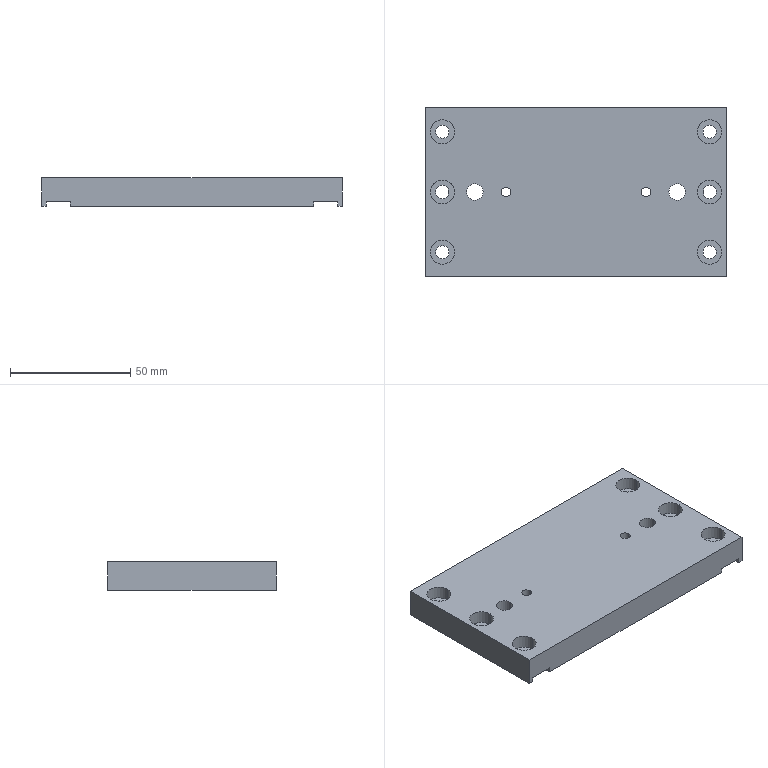Part | STEP file | C05 | 1 solid | 52 faces | box 125 x 70 x 12 mm | volume 97826 mm3 | cylinder 32 | plane 20 | commonest cylinder face diameters 5.5 x12 10 x12 4 x4 6.8 x4